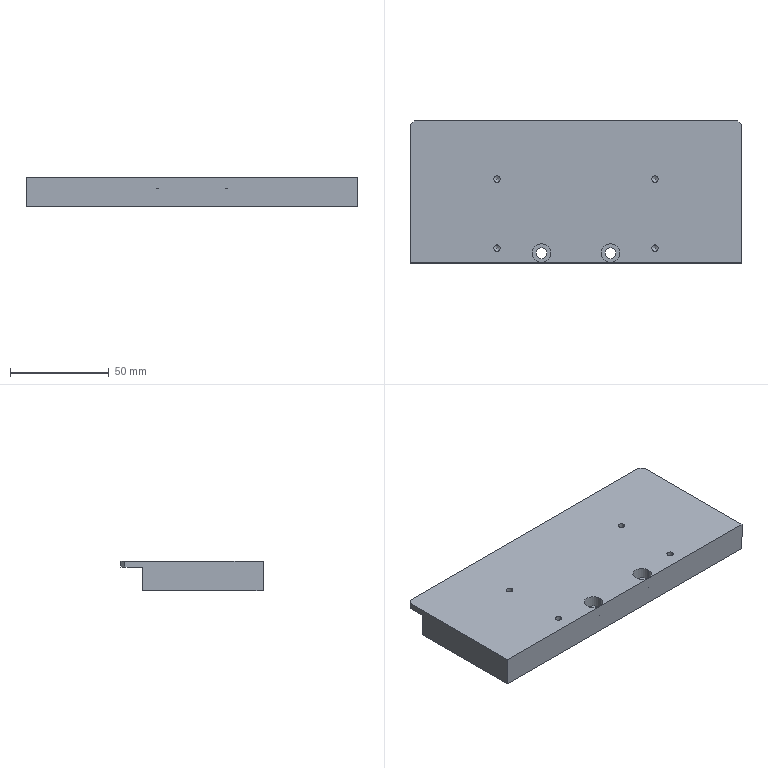Part | SolidWorks | features HoleWzd 10, ICE 4, Chamfer 2, Cut 1, Extrusion 1, Fillet 1 | 1 solid | 52 faces | box 168 x 72 x 15 mm | volume 156428 mm3 | cylinder 24 | cone 16 | plane 12 | commonest cylinder face diameters 3.3 x8 5 x8 5.5 x4 9.5 x4
STEP:
#1=CARTESIAN_POINT('',(61.75,272.,1.8));
#2=VERTEX_POINT('',#1);
#3=CARTESIAN_POINT('',(71.25,272.,1.8));
#4=VERTEX_POINT('',#3);
#5=CARTESIAN_POINT('',(66.5,272.,1.8));
#6=DIRECTION('',(0.,0.,1.));
#7=DIRECTION('',(1.,0.,0.));
#8=AXIS2_PLACEMENT_3D('',#5,#6,#7);
#9=CIRCLE('',#8,4.75);
#10=EDGE_CURVE('',#2,#4,#9,.T.);
#11=ORIENTED_EDGE('',*,*,#10,.F.);
#12=CARTESIAN_POINT('',(61.75,272.,7.5));
#13=VERTEX_POINT('',#12);
#14=CARTESIAN_POINT('',(61.75,272.,7.5));
#15=DIRECTION('',(0.,0.,1.));
#16=VECTOR('',#15,1000.);
#17=LINE('',#14,#16);
#18=EDGE_CURVE('',#2,#13,#17,.T.);
#19=ORIENTED_EDGE('',*,*,#18,.T.);
#20=CARTESIAN_POINT('',(71.25,272.,7.5));
#21=VERTEX_POINT('',#20);
#22=CARTESIAN_POINT('',(66.5,272.,7.5));
#23=DIRECTION('',(0.,0.,1.));
#24=DIRECTION('',(1.,0.,0.));
#25=AXIS2_PLACEMENT_3D('',#22,#23,#24);
#26=CIRCLE('',#25,4.75);
#27=EDGE_CURVE('',#13,#21,#26,.T.);
#28=ORIENTED_EDGE('',*,*,#27,.T.);
#29=CARTESIAN_POINT('',(71.25,272.,7.5));
#30=DIRECTION('',(0.,0.,1.));
#31=VECTOR('',#30,1000.);
#32=LINE('',#29,#31);
#33=EDGE_CURVE('',#4,#21,#32,.T.);
#34=ORIENTED_EDGE('',*,*,#33,.F.);
#35=EDGE_LOOP('',(#11,#19,#28,#34));
#36=FACE_OUTER_BOUND('',#35,.T.);
#37=CARTESIAN_POINT('',(66.5,272.,7.5));
#38=DIRECTION('',(0.,0.,1.));
#39=DIRECTION('',(1.,0.,0.));
#40=AXIS2_PLACEMENT_3D('',#37,#38,#39);
#41=CYLINDRICAL_SURFACE('',#40,4.75);
#42=ADVANCED_FACE('',(#36),#41,.F.);
#43=CARTESIAN_POINT('',(63.75,272.,-7.5));
#44=VERTEX_POINT('',#43);
#45=CARTESIAN_POINT('',(69.25,272.,-7.5));
#46=VERTEX_POINT('',#45);
#47=CARTESIAN_POINT('',(66.5,272.,-7.5));
#48=DIRECTION('',(0.,0.,1.));
#49=DIRECTION('',(1.,0.,0.));
#50=AXIS2_PLACEMENT_3D('',#47,#48,#49);
#51=CIRCLE('',#50,2.75);
#52=EDGE_CURVE('',#44,#46,#51,.T.);
#53=ORIENTED_EDGE('',*,*,#52,.F.);
#54=CARTESIAN_POINT('',(63.75,272.,1.8));
#55=VERTEX_POINT('',#54);
#56=CARTESIAN_POINT('',(63.75,272.,7.5));
#57=DIRECTION('',(0.,0.,1.));
#58=VECTOR('',#57,1000.);
#59=LINE('',#56,#58);
#60=EDGE_CURVE('',#44,#55,#59,.T.);
#61=ORIENTED_EDGE('',*,*,#60,.T.);
#62=CARTESIAN_POINT('',(69.25,272.,1.8));
#63=VERTEX_POINT('',#62);
#64=CARTESIAN_POINT('',(66.5,272.,1.8));
#65=DIRECTION('',(0.,0.,1.));
#66=DIRECTION('',(1.,0.,0.));
#67=AXIS2_PLACEMENT_3D('',#64,#65,#66);
#68=CIRCLE('',#67,2.75);
#69=EDGE_CURVE('',#55,#63,#68,.T.);
#70=ORIENTED_EDGE('',*,*,#69,.T.);
#71=CARTESIAN_POINT('',(69.25,272.,7.5));
#72=DIRECTION('',(0.,0.,1.));
#73=VECTOR('',#72,1000.);
#74=LINE('',#71,#73);
#75=EDGE_CURVE('',#46,#63,#74,.T.);
#76=ORIENTED_EDGE('',*,*,#75,.F.);
#77=EDGE_LOOP('',(#53,#61,#70,#76));
#78=FACE_OUTER_BOUND('',#77,.T.);
#79=CARTESIAN_POINT('',(66.5,272.,7.5));
#80=DIRECTION('',(0.,0.,1.));
#81=DIRECTION('',(1.,0.,0.));
#82=AXIS2_PLACEMENT_3D('',#79,#80,#81);
#83=CYLINDRICAL_SURFACE('',#82,2.75);
#84=ADVANCED_FACE('',(#78),#83,.F.);
#85=CARTESIAN_POINT('',(96.75,272.,1.8));
#86=VERTEX_POINT('',#85);
#87=CARTESIAN_POINT('',(106.25,272.,1.8));
#88=VERTEX_POINT('',#87);
#89=CARTESIAN_POINT('',(101.5,272.,1.8));
#90=DIRECTION('',(0.,0.,1.));
#91=DIRECTION('',(1.,0.,0.));
#92=AXIS2_PLACEMENT_3D('',#89,#90,#91);
#93=CIRCLE('',#92,4.75);
#94=EDGE_CURVE('',#86,#88,#93,.T.);
#95=ORIENTED_EDGE('',*,*,#94,.F.);
#96=CARTESIAN_POINT('',(96.75,272.,7.5));
#97=VERTEX_POINT('',#96);
#98=CARTESIAN_POINT('',(96.75,272.,7.5));
#99=DIRECTION('',(0.,0.,1.));
#100=VECTOR('',#99,1000.);
#101=LINE('',#98,#100);
#102=EDGE_CURVE('',#86,#97,#101,.T.);
#103=ORIENTED_EDGE('',*,*,#102,.T.);
#104=CARTESIAN_POINT('',(106.25,272.,7.5));
#105=VERTEX_POINT('',#104);
#106=CARTESIAN_POINT('',(101.5,272.,7.5));
#107=DIRECTION('',(0.,0.,1.));
#108=DIRECTION('',(1.,0.,0.));
#109=AXIS2_PLACEMENT_3D('',#106,#107,#108);
#110=CIRCLE('',#109,4.75);
#111=EDGE_CURVE('',#97,#105,#110,.T.);
#112=ORIENTED_EDGE('',*,*,#111,.T.);
#113=CARTESIAN_POINT('',(106.25,272.,7.5));
#114=DIRECTION('',(0.,0.,1.));
#115=VECTOR('',#114,1000.);
#116=LINE('',#113,#115);
#117=EDGE_CURVE('',#88,#105,#116,.T.);
#118=ORIENTED_EDGE('',*,*,#117,.F.);
#119=EDGE_LOOP('',(#95,#103,#112,#118));
#120=FACE_OUTER_BOUND('',#119,.T.);
#121=CARTESIAN_POINT('',(101.5,272.,7.5));
#122=DIRECTION('',(0.,0.,1.));
#123=DIRECTION('',(1.,0.,0.));
#124=AXIS2_PLACEMENT_3D('',#121,#122,#123);
#125=CYLINDRICAL_SURFACE('',#124,4.75);
#126=ADVANCED_FACE('',(#120),#125,.F.);
#127=CARTESIAN_POINT('',(98.75,272.,-7.5));
#128=VERTEX_POINT('',#127);
#129=CARTESIAN_POINT('',(104.25,272.,-7.5));
#130=VERTEX_POINT('',#129);
#131=CARTESIAN_POINT('',(101.5,272.,-7.5));
#132=DIRECTION('',(0.,0.,1.));
#133=DIRECTION('',(1.,0.,0.));
#134=AXIS2_PLACEMENT_3D('',#131,#132,#133);
#135=CIRCLE('',#134,2.75);
#136=EDGE_CURVE('',#128,#130,#135,.T.);
#137=ORIENTED_EDGE('',*,*,#136,.F.);
#138=CARTESIAN_POINT('',(98.75,272.,1.8));
#139=VERTEX_POINT('',#138);
#140=CARTESIAN_POINT('',(98.75,272.,7.5));
#141=DIRECTION('',(0.,0.,1.));
#142=VECTOR('',#141,1000.);
#143=LINE('',#140,#142);
#144=EDGE_CURVE('',#128,#139,#143,.T.);
#145=ORIENTED_EDGE('',*,*,#144,.T.);
#146=CARTESIAN_POINT('',(104.25,272.,1.8));
#147=VERTEX_POINT('',#146);
#148=CARTESIAN_POINT('',(101.5,272.,1.8));
#149=DIRECTION('',(0.,0.,1.));
#150=DIRECTION('',(1.,0.,0.));
#151=AXIS2_PLACEMENT_3D('',#148,#149,#150);
#152=CIRCLE('',#151,2.75);
#153=EDGE_CURVE('',#139,#147,#152,.T.);
#154=ORIENTED_EDGE('',*,*,#153,.T.);
#155=CARTESIAN_POINT('',(104.25,272.,7.5));
#156=DIRECTION('',(0.,0.,1.));
#157=VECTOR('',#156,1000.);
#158=LINE('',#155,#157);
#159=EDGE_CURVE('',#130,#147,#158,.T.);
#160=ORIENTED_EDGE('',*,*,#159,.F.);
#161=EDGE_LOOP('',(#137,#145,#154,#160));
#162=FACE_OUTER_BOUND('',#161,.T.);
#163=CARTESIAN_POINT('',(101.5,272.,7.5));
#164=DIRECTION('',(0.,0.,1.));
#165=DIRECTION('',(1.,0.,0.));
#166=AXIS2_PLACEMENT_3D('',#163,#164,#165);
#167=CYLINDRICAL_SURFACE('',#166,2.75);
#168=ADVANCED_FACE('',(#162),#167,.F.);
#169=CARTESIAN_POINT('',(42.35,309.5,-2.6));
#170=VERTEX_POINT('',#169);
#171=CARTESIAN_POINT('',(45.65,309.5,-2.6));
#172=VERTEX_POINT('',#171);
#173=CARTESIAN_POINT('',(44.,309.5,-2.6));
#174=DIRECTION('',(0.,0.,1.));
#175=DIRECTION('',(1.,0.,0.));
#176=AXIS2_PLACEMENT_3D('',#173,#174,#175);
#177=CIRCLE('',#176,1.65);
#178=EDGE_CURVE('',#170,#172,#177,.T.);
#179=ORIENTED_EDGE('',*,*,#178,.F.);
#180=CARTESIAN_POINT('',(42.35,309.5,7.5));
#181=VERTEX_POINT('',#180);
#182=CARTESIAN_POINT('',(42.35,309.5,7.5));
#183=DIRECTION('',(0.,0.,1.));
#184=VECTOR('',#183,1000.);
#185=LINE('',#182,#184);
#186=EDGE_CURVE('',#170,#181,#185,.T.);
#187=ORIENTED_EDGE('',*,*,#186,.T.);
#188=CARTESIAN_POINT('',(45.65,309.5,7.5));
#189=VERTEX_POINT('',#188);
#190=CARTESIAN_POINT('',(44.,309.5,7.5));
#191=DIRECTION('',(0.,0.,1.));
#192=DIRECTION('',(1.,0.,0.));
#193=AXIS2_PLACEMENT_3D('',#190,#191,#192);
#194=CIRCLE('',#193,1.65);
#195=EDGE_CURVE('',#181,#189,#194,.T.);
#196=ORIENTED_EDGE('',*,*,#195,.T.);
#197=CARTESIAN_POINT('',(45.65,309.5,7.5));
#198=DIRECTION('',(0.,0.,1.));
#199=VECTOR('',#198,1000.);
#200=LINE('',#197,#199);
#201=EDGE_CURVE('',#172,#189,#200,.T.);
#202=ORIENTED_EDGE('',*,*,#201,.F.);
#203=EDGE_LOOP('',(#179,#187,#196,#202));
#204=FACE_OUTER_BOUND('',#203,.T.);
#205=CARTESIAN_POINT('',(44.,309.5,7.5));
#206=DIRECTION('',(0.,0.,1.));
#207=DIRECTION('',(1.,0.,0.));
#208=AXIS2_PLACEMENT_3D('',#205,#206,#207);
#209=CYLINDRICAL_SURFACE('',#208,1.65);
#210=ADVANCED_FACE('',(#204),#209,.F.);
#211=CARTESIAN_POINT('',(44.,309.5,-3.591));
#212=VERTEX_POINT('',#211);
#213=CARTESIAN_POINT('',(45.65,309.5,-2.6));
#214=DIRECTION('',(0.8572,0.,0.515));
#215=VECTOR('',#214,1000.);
#216=LINE('',#213,#215);
#217=EDGE_CURVE('',#212,#172,#216,.T.);
#218=ORIENTED_EDGE('',*,*,#217,.F.);
#219=CARTESIAN_POINT('',(42.35,309.5,-2.6));
#220=DIRECTION('',(-0.8572,0.,0.515));
#221=VECTOR('',#220,1000.);
#222=LINE('',#219,#221);
#223=EDGE_CURVE('',#212,#170,#222,.T.);
#224=ORIENTED_EDGE('',*,*,#223,.T.);
#225=ORIENTED_EDGE('',*,*,#178,.T.);
#226=EDGE_LOOP('',(#218,#224,#225));
#227=FACE_OUTER_BOUND('',#226,.T.);
#228=CARTESIAN_POINT('',(44.,309.5,-2.6));
#229=DIRECTION('',(0.,0.,1.));
#230=DIRECTION('',(1.,0.,0.));
#231=AXIS2_PLACEMENT_3D('',#228,#229,#230);
#232=CONICAL_SURFACE('',#231,1.65,1.03);
#233=ADVANCED_FACE('',(#227),#232,.F.);
#234=CARTESIAN_POINT('',(42.35,274.5,-2.6));
#235=VERTEX_POINT('',#234);
#236=CARTESIAN_POINT('',(45.65,274.5,-2.6));
#237=VERTEX_POINT('',#236);
#238=CARTESIAN_POINT('',(44.,274.5,-2.6));
#239=DIRECTION('',(0.,0.,1.));
#240=DIRECTION('',(1.,0.,0.));
#241=AXIS2_PLACEMENT_3D('',#238,#239,#240);
#242=CIRCLE('',#241,1.65);
#243=EDGE_CURVE('',#235,#237,#242,.T.);
#244=ORIENTED_EDGE('',*,*,#243,.F.);
#245=CARTESIAN_POINT('',(42.35,274.5,7.5));
#246=VERTEX_POINT('',#245);
#247=CARTESIAN_POINT('',(42.35,274.5,7.5));
#248=DIRECTION('',(0.,0.,1.));
#249=VECTOR('',#248,1000.);
#250=LINE('',#247,#249);
#251=EDGE_CURVE('',#235,#246,#250,.T.);
#252=ORIENTED_EDGE('',*,*,#251,.T.);
#253=CARTESIAN_POINT('',(45.65,274.5,7.5));
#254=VERTEX_POINT('',#253);
#255=CARTESIAN_POINT('',(44.,274.5,7.5));
#256=DIRECTION('',(0.,0.,1.));
#257=DIRECTION('',(1.,0.,0.));
#258=AXIS2_PLACEMENT_3D('',#255,#256,#257);
#259=CIRCLE('',#258,1.65);
#260=EDGE_CURVE('',#246,#254,#259,.T.);
#261=ORIENTED_EDGE('',*,*,#260,.T.);
#262=CARTESIAN_POINT('',(45.65,274.5,7.5));
#263=DIRECTION('',(0.,0.,1.));
#264=VECTOR('',#263,1000.);
#265=LINE('',#262,#264);
#266=EDGE_CURVE('',#237,#254,#265,.T.);
#267=ORIENTED_EDGE('',*,*,#266,.F.);
#268=EDGE_LOOP('',(#244,#252,#261,#267));
#269=FACE_OUTER_BOUND('',#268,.T.);
#270=CARTESIAN_POINT('',(44.,274.5,7.5));
#271=DIRECTION('',(0.,0.,1.));
#272=DIRECTION('',(1.,0.,0.));
#273=AXIS2_PLACEMENT_3D('',#270,#271,#272);
#274=CYLINDRICAL_SURFACE('',#273,1.65);
#275=ADVANCED_FACE('',(#269),#274,.F.);
#276=CARTESIAN_POINT('',(44.,274.5,-3.591));
#277=VERTEX_POINT('',#276);
#278=CARTESIAN_POINT('',(45.65,274.5,-2.6));
#279=DIRECTION('',(0.8572,0.,0.515));
#280=VECTOR('',#279,1000.);
#281=LINE('',#278,#280);
#282=EDGE_CURVE('',#277,#237,#281,.T.);
#283=ORIENTED_EDGE('',*,*,#282,.F.);
#284=CARTESIAN_POINT('',(42.35,274.5,-2.6));
#285=DIRECTION('',(-0.8572,0.,0.515));
#286=VECTOR('',#285,1000.);
#287=LINE('',#284,#286);
#288=EDGE_CURVE('',#277,#235,#287,.T.);
#289=ORIENTED_EDGE('',*,*,#288,.T.);
#290=ORIENTED_EDGE('',*,*,#243,.T.);
#291=EDGE_LOOP('',(#283,#289,#290));
#292=FACE_OUTER_BOUND('',#291,.T.);
#293=CARTESIAN_POINT('',(44.,274.5,-2.6));
#294=DIRECTION('',(0.,0.,1.));
#295=DIRECTION('',(1.,0.,0.));
#296=AXIS2_PLACEMENT_3D('',#293,#294,#295);
#297=CONICAL_SURFACE('',#296,1.65,1.03);
#298=ADVANCED_FACE('',(#292),#297,.F.);
#299=CARTESIAN_POINT('',(122.35,274.5,-2.6));
#300=VERTEX_POINT('',#299);
#301=CARTESIAN_POINT('',(125.65,274.5,-2.6));
#302=VERTEX_POINT('',#301);
#303=CARTESIAN_POINT('',(124.,274.5,-2.6));
#304=DIRECTION('',(0.,0.,1.));
#305=DIRECTION('',(1.,0.,0.));
#306=AXIS2_PLACEMENT_3D('',#303,#304,#305);
#307=CIRCLE('',#306,1.65);
#308=EDGE_CURVE('',#300,#302,#307,.T.);
#309=ORIENTED_EDGE('',*,*,#308,.F.);
#310=CARTESIAN_POINT('',(122.35,274.5,7.5));
#311=VERTEX_POINT('',#310);
#312=CARTESIAN_POINT('',(122.35,274.5,7.5));
#313=DIRECTION('',(0.,0.,1.));
#314=VECTOR('',#313,1000.);
#315=LINE('',#312,#314);
#316=EDGE_CURVE('',#300,#311,#315,.T.);
#317=ORIENTED_EDGE('',*,*,#316,.T.);
#318=CARTESIAN_POINT('',(125.65,274.5,7.5));
#319=VERTEX_POINT('',#318);
#320=CARTESIAN_POINT('',(124.,274.5,7.5));
#321=DIRECTION('',(0.,0.,1.));
#322=DIRECTION('',(1.,0.,0.));
#323=AXIS2_PLACEMENT_3D('',#320,#321,#322);
#324=CIRCLE('',#323,1.65);
#325=EDGE_CURVE('',#311,#319,#324,.T.);
#326=ORIENTED_EDGE('',*,*,#325,.T.);
#327=CARTESIAN_POINT('',(125.65,274.5,7.5));
#328=DIRECTION('',(0.,0.,1.));
#329=VECTOR('',#328,1000.);
#330=LINE('',#327,#329);
#331=EDGE_CURVE('',#302,#319,#330,.T.);
#332=ORIENTED_EDGE('',*,*,#331,.F.);
#333=EDGE_LOOP('',(#309,#317,#326,#332));
#334=FACE_OUTER_BOUND('',#333,.T.);
#335=CARTESIAN_POINT('',(124.,274.5,7.5));
#336=DIRECTION('',(0.,0.,1.));
#337=DIRECTION('',(1.,0.,0.));
#338=AXIS2_PLACEMENT_3D('',#335,#336,#337);
#339=CYLINDRICAL_SURFACE('',#338,1.65);
#340=ADVANCED_FACE('',(#334),#339,.F.);
#341=CARTESIAN_POINT('',(124.,274.5,-3.591));
#342=VERTEX_POINT('',#341);
#343=CARTESIAN_POINT('',(125.65,274.5,-2.6));
#344=DIRECTION('',(0.8572,0.,0.515));
#345=VECTOR('',#344,1000.);
#346=LINE('',#343,#345);
#347=EDGE_CURVE('',#342,#302,#346,.T.);
#348=ORIENTED_EDGE('',*,*,#347,.F.);
#349=CARTESIAN_POINT('',(122.35,274.5,-2.6));
#350=DIRECTION('',(-0.8572,0.,0.515));
#351=VECTOR('',#350,1000.);
#352=LINE('',#349,#351);
#353=EDGE_CURVE('',#342,#300,#352,.T.);
#354=ORIENTED_EDGE('',*,*,#353,.T.);
#355=ORIENTED_EDGE('',*,*,#308,.T.);
#356=EDGE_LOOP('',(#348,#354,#355));
#357=FACE_OUTER_BOUND('',#356,.T.);
#358=CARTESIAN_POINT('',(124.,274.5,-2.6));
#359=DIRECTION('',(0.,0.,1.));
#360=DIRECTION('',(1.,0.,0.));
#361=AXIS2_PLACEMENT_3D('',#358,#359,#360);
#362=CONICAL_SURFACE('',#361,1.65,1.03);
#363=ADVANCED_FACE('',(#357),#362,.F.);
#364=CARTESIAN_POINT('',(122.35,309.5,-2.6));
#365=VERTEX_POINT('',#364);
#366=CARTESIAN_POINT('',(125.65,309.5,-2.6));
#367=VERTEX_POINT('',#366);
#368=CARTESIAN_POINT('',(124.,309.5,-2.6));
#369=DIRECTION('',(0.,0.,1.));
#370=DIRECTION('',(1.,0.,0.));
#371=AXIS2_PLACEMENT_3D('',#368,#369,#370);
#372=CIRCLE('',#371,1.65);
#373=EDGE_CURVE('',#365,#367,#372,.T.);
#374=ORIENTED_EDGE('',*,*,#373,.F.);
#375=CARTESIAN_POINT('',(122.35,309.5,7.5));
#376=VERTEX_POINT('',#375);
#377=CARTESIAN_POINT('',(122.35,309.5,7.5));
#378=DIRECTION('',(0.,0.,1.));
#379=VECTOR('',#378,1000.);
#380=LINE('',#377,#379);
#381=EDGE_CURVE('',#365,#376,#380,.T.);
#382=ORIENTED_EDGE('',*,*,#381,.T.);
#383=CARTESIAN_POINT('',(125.65,309.5,7.5));
#384=VERTEX_POINT('',#383);
#385=CARTESIAN_POINT('',(124.,309.5,7.5));
#386=DIRECTION('',(0.,0.,1.));
#387=DIRECTION('',(1.,0.,0.));
#388=AXIS2_PLACEMENT_3D('',#385,#386,#387);
#389=CIRCLE('',#388,1.65);
#390=EDGE_CURVE('',#376,#384,#389,.T.);
#391=ORIENTED_EDGE('',*,*,#390,.T.);
#392=CARTESIAN_POINT('',(125.65,309.5,7.5));
#393=DIRECTION('',(0.,0.,1.));
#394=VECTOR('',#393,1000.);
#395=LINE('',#392,#394);
#396=EDGE_CURVE('',#367,#384,#395,.T.);
#397=ORIENTED_EDGE('',*,*,#396,.F.);
#398=EDGE_LOOP('',(#374,#382,#391,#397));
#399=FACE_OUTER_BOUND('',#398,.T.);
#400=CARTESIAN_POINT('',(124.,309.5,7.5));
#401=DIRECTION('',(0.,0.,1.));
#402=DIRECTION('',(1.,0.,0.));
#403=AXIS2_PLACEMENT_3D('',#400,#401,#402);
#404=CYLINDRICAL_SURFACE('',#403,1.65);
#405=ADVANCED_FACE('',(#399),#404,.F.);
#406=CARTESIAN_POINT('',(124.,309.5,-3.591));
#407=VERTEX_POINT('',#406);
#408=CARTESIAN_POINT('',(125.65,309.5,-2.6));
#409=DIRECTION('',(0.8572,0.,0.515));
#410=VECTOR('',#409,1000.);
#411=LINE('',#408,#410);
#412=EDGE_CURVE('',#407,#367,#411,.T.);
#413=ORIENTED_EDGE('',*,*,#412,.F.);
#414=CARTESIAN_POINT('',(122.35,309.5,-2.6));
#415=DIRECTION('',(-0.8572,0.,0.515));
#416=VECTOR('',#415,1000.);
#417=LINE('',#414,#416);
#418=EDGE_CURVE('',#407,#365,#417,.T.);
#419=ORIENTED_EDGE('',*,*,#418,.T.);
#420=ORIENTED_EDGE('',*,*,#373,.T.);
#421=EDGE_LOOP('',(#413,#419,#420));
#422=FACE_OUTER_BOUND('',#421,.T.);
#423=CARTESIAN_POINT('',(124.,309.5,-2.6));
#424=DIRECTION('',(0.,0.,1.));
#425=DIRECTION('',(1.,0.,0.));
#426=AXIS2_PLACEMENT_3D('',#423,#424,#425);
#427=CONICAL_SURFACE('',#426,1.65,1.03);
#428=ADVANCED_FACE('',(#422),#427,.F.);
#429=CARTESIAN_POINT('',(151.5,313.,-4.));
#430=VERTEX_POINT('',#429);
#431=CARTESIAN_POINT('',(151.5,313.,1.));
#432=VERTEX_POINT('',#431);
#433=CARTESIAN_POINT('',(151.5,313.,-1.5));
#434=DIRECTION('',(0.,1.,0.));
#435=DIRECTION('',(0.,0.,1.));
#436=AXIS2_PLACEMENT_3D('',#433,#434,#435);
#437=CIRCLE('',#436,2.5);
#438=EDGE_CURVE('',#430,#432,#437,.T.);
#439=ORIENTED_EDGE('',*,*,#438,.F.);
#440=CARTESIAN_POINT('',(151.5,328.,-4.));
#441=VERTEX_POINT('',#440);
#442=CARTESIAN_POINT('',(151.5,328.,-4.));
#443=DIRECTION('',(0.,1.,0.));
#444=VECTOR('',#443,1000.);
#445=LINE('',#442,#444);
#446=EDGE_CURVE('',#430,#441,#445,.T.);
#447=ORIENTED_EDGE('',*,*,#446,.T.);
#448=CARTESIAN_POINT('',(151.5,328.,1.));
#449=VERTEX_POINT('',#448);
#450=CARTESIAN_POINT('',(151.5,328.,-1.5));
#451=DIRECTION('',(0.,1.,0.));
#452=DIRECTION('',(0.,0.,1.));
#453=AXIS2_PLACEMENT_3D('',#450,#451,#452);
#454=CIRCLE('',#453,2.5);
#455=EDGE_CURVE('',#441,#449,#454,.T.);
#456=ORIENTED_EDGE('',*,*,#455,.T.);
#457=CARTESIAN_POINT('',(151.5,328.,1.));
#458=DIRECTION('',(0.,1.,0.));
#459=VECTOR('',#458,1000.);
#460=LINE('',#457,#459);
#461=EDGE_CURVE('',#432,#449,#460,.T.);
#462=ORIENTED_EDGE('',*,*,#461,.F.);
#463=EDGE_LOOP('',(#439,#447,#456,#462));
#464=FACE_OUTER_BOUND('',#463,.T.);
#465=CARTESIAN_POINT('',(151.5,328.,-1.5));
#466=DIRECTION('',(0.,1.,0.));
#467=DIRECTION('',(0.,0.,1.));
#468=AXIS2_PLACEMENT_3D('',#465,#466,#467);
#469=CYLINDRICAL_SURFACE('',#468,2.5);
#470=ADVANCED_FACE('',(#464),#469,.F.);
#471=CARTESIAN_POINT('',(151.5,311.498,-1.5));
#472=VERTEX_POINT('',#471);
#473=CARTESIAN_POINT('',(151.5,313.,1.));
#474=DIRECTION('',(0.,0.515,0.8572));
#475=VECTOR('',#474,1000.);
#476=LINE('',#473,#475);
#477=EDGE_CURVE('',#472,#432,#476,.T.);
#478=ORIENTED_EDGE('',*,*,#477,.F.);
#479=CARTESIAN_POINT('',(151.5,313.,-4.));
#480=DIRECTION('',(0.,0.515,-0.8572));
#481=VECTOR('',#480,1000.);
#482=LINE('',#479,#481);
#483=EDGE_CURVE('',#472,#430,#482,.T.);
#484=ORIENTED_EDGE('',*,*,#483,.T.);
#485=ORIENTED_EDGE('',*,*,#438,.T.);
#486=EDGE_LOOP('',(#478,#484,#485));
#487=FACE_OUTER_BOUND('',#486,.T.);
#488=CARTESIAN_POINT('',(151.5,313.,-1.5));
#489=DIRECTION('',(0.,1.,0.));
#490=DIRECTION('',(0.,0.,1.));
#491=AXIS2_PLACEMENT_3D('',#488,#489,#490);
#492=CONICAL_SURFACE('',#491,2.5,1.03);
#493=ADVANCED_FACE('',(#487),#492,.F.);
#494=CARTESIAN_POINT('',(106.5,313.,-4.));
#495=VERTEX_POINT('',#494);
#496=CARTESIAN_POINT('',(106.5,313.,1.));
#497=VERTEX_POINT('',#496);
#498=CARTESIAN_POINT('',(106.5,313.,-1.5));
#499=DIRECTION('',(0.,1.,0.));
#500=DIRECTION('',(0.,0.,1.));
#501=AXIS2_PLACEMENT_3D('',#498,#499,#500);
#502=CIRCLE('',#501,2.5);
#503=EDGE_CURVE('',#495,#497,#502,.T.);
#504=ORIENTED_EDGE('',*,*,#503,.F.);
#505=CARTESIAN_POINT('',(106.5,328.,-4.));
#506=VERTEX_POINT('',#505);
#507=CARTESIAN_POINT('',(106.5,328.,-4.));
#508=DIRECTION('',(0.,1.,0.));
#509=VECTOR('',#508,1000.);
#510=LINE('',#507,#509);
#511=EDGE_CURVE('',#495,#506,#510,.T.);
#512=ORIENTED_EDGE('',*,*,#511,.T.);
#513=CARTESIAN_POINT('',(106.5,328.,1.));
#514=VERTEX_POINT('',#513);
#515=CARTESIAN_POINT('',(106.5,328.,-1.5));
#516=DIRECTION('',(0.,1.,0.));
#517=DIRECTION('',(0.,0.,1.));
#518=AXIS2_PLACEMENT_3D('',#515,#516,#517);
#519=CIRCLE('',#518,2.5);
#520=EDGE_CURVE('',#506,#514,#519,.T.);
#521=ORIENTED_EDGE('',*,*,#520,.T.);
#522=CARTESIAN_POINT('',(106.5,328.,1.));
#523=DIRECTION('',(0.,1.,0.));
#524=VECTOR('',#523,1000.);
#525=LINE('',#522,#524);
#526=EDGE_CURVE('',#497,#514,#525,.T.);
#527=ORIENTED_EDGE('',*,*,#526,.F.);
#528=EDGE_LOOP('',(#504,#512,#521,#527));
#529=FACE_OUTER_BOUND('',#528,.T.);
#530=CARTESIAN_POINT('',(106.5,328.,-1.5));
#531=DIRECTION('',(0.,1.,0.));
#532=DIRECTION('',(0.,0.,1.));
#533=AXIS2_PLACEMENT_3D('',#530,#531,#532);
#534=CYLINDRICAL_SURFACE('',#533,2.5);
#535=ADVANCED_FACE('',(#529),#534,.F.);
#536=CARTESIAN_POINT('',(106.5,311.498,-1.5));
#537=VERTEX_POINT('',#536);
#538=CARTESIAN_POINT('',(106.5,313.,1.));
#539=DIRECTION('',(0.,0.515,0.8572));
#540=VECTOR('',#539,1000.);
#541=LINE('',#538,#540);
#542=EDGE_CURVE('',#537,#497,#541,.T.);
#543=ORIENTED_EDGE('',*,*,#542,.F.);
#544=CARTESIAN_POINT('',(106.5,313.,-4.));
#545=DIRECTION('',(0.,0.515,-0.8572));
#546=VECTOR('',#545,1000.);
#547=LINE('',#544,#546);
#548=EDGE_CURVE('',#537,#495,#547,.T.);
#549=ORIENTED_EDGE('',*,*,#548,.T.);
#550=ORIENTED_EDGE('',*,*,#503,.T.);
#551=EDGE_LOOP('',(#543,#549,#550));
#552=FACE_OUTER_BOUND('',#551,.T.);
#553=CARTESIAN_POINT('',(106.5,313.,-1.5));
#554=DIRECTION('',(0.,1.,0.));
#555=DIRECTION('',(0.,0.,1.));
#556=AXIS2_PLACEMENT_3D('',#553,#554,#555);
#557=CONICAL_SURFACE('',#556,2.5,1.03);
#558=ADVANCED_FACE('',(#552),#557,.F.);
#559=CARTESIAN_POINT('',(61.5,313.,-4.));
#560=VERTEX_POINT('',#559);
#561=CARTESIAN_POINT('',(61.5,313.,1.));
#562=VERTEX_POINT('',#561);
#563=CARTESIAN_POINT('',(61.5,313.,-1.5));
#564=DIRECTION('',(0.,1.,0.));
#565=DIRECTION('',(0.,0.,1.));
#566=AXIS2_PLACEMENT_3D('',#563,#564,#565);
#567=CIRCLE('',#566,2.5);
#568=EDGE_CURVE('',#560,#562,#567,.T.);
#569=ORIENTED_EDGE('',*,*,#568,.F.);
#570=CARTESIAN_POINT('',(61.5,328.,-4.));
#571=VERTEX_POINT('',#570);
#572=CARTESIAN_POINT('',(61.5,328.,-4.));
#573=DIRECTION('',(0.,1.,0.));
#574=VECTOR('',#573,1000.);
#575=LINE('',#572,#574);
#576=EDGE_CURVE('',#560,#571,#575,.T.);
#577=ORIENTED_EDGE('',*,*,#576,.T.);
#578=CARTESIAN_POINT('',(61.5,328.,1.));
#579=VERTEX_POINT('',#578);
#580=CARTESIAN_POINT('',(61.5,328.,-1.5));
#581=DIRECTION('',(0.,1.,0.));
#582=DIRECTION('',(0.,0.,1.));
#583=AXIS2_PLACEMENT_3D('',#580,#581,#582);
#584=CIRCLE('',#583,2.5);
#585=EDGE_CURVE('',#571,#579,#584,.T.);
#586=ORIENTED_EDGE('',*,*,#585,.T.);
#587=CARTESIAN_POINT('',(61.5,328.,1.));
#588=DIRECTION('',(0.,1.,0.));
#589=VECTOR('',#588,1000.);
#590=LINE('',#587,#589);
#591=EDGE_CURVE('',#562,#579,#590,.T.);
#592=ORIENTED_EDGE('',*,*,#591,.F.);
#593=EDGE_LOOP('',(#569,#577,#586,#592));
#594=FACE_OUTER_BOUND('',#593,.T.);
#595=CARTESIAN_POINT('',(61.5,328.,-1.5));
#596=DIRECTION('',(0.,1.,0.));
#597=DIRECTION('',(0.,0.,1.));
#598=AXIS2_PLACEMENT_3D('',#595,#596,#597);
#599=CYLINDRICAL_SURFACE('',#598,2.5);
#600=ADVANCED_FACE('',(#594),#599,.F.);
#601=CARTESIAN_POINT('',(61.5,311.498,-1.5));
#602=VERTEX_POINT('',#601);
#603=CARTESIAN_POINT('',(61.5,313.,1.));
#604=DIRECTION('',(0.,0.515,0.8572));
#605=VECTOR('',#604,1000.);
#606=LINE('',#603,#605);
#607=EDGE_CURVE('',#602,#562,#606,.T.);
#608=ORIENTED_EDGE('',*,*,#607,.F.);
#609=CARTESIAN_POINT('',(61.5,313.,-4.));
#610=DIRECTION('',(0.,0.515,-0.8572));
#611=VECTOR('',#610,1000.);
#612=LINE('',#609,#611);
#613=EDGE_CURVE('',#602,#560,#612,.T.);
#614=ORIENTED_EDGE('',*,*,#613,.T.);
#615=ORIENTED_EDGE('',*,*,#568,.T.);
#616=EDGE_LOOP('',(#608,#614,#615));
#617=FACE_OUTER_BOUND('',#616,.T.);
#618=CARTESIAN_POINT('',(61.5,313.,-1.5));
#619=DIRECTION('',(0.,1.,0.));
#620=DIRECTION('',(0.,0.,1.));
#621=AXIS2_PLACEMENT_3D('',#618,#619,#620);
#622=CONICAL_SURFACE('',#621,2.5,1.03);
#623=ADVANCED_FACE('',(#617),#622,.F.);
#624=CARTESIAN_POINT('',(16.5,313.,-4.));
#625=VERTEX_POINT('',#624);
#626=CARTESIAN_POINT('',(16.5,313.,1.));
#627=VERTEX_POINT('',#626);
#628=CARTESIAN_POINT('',(16.5,313.,-1.5));
#629=DIRECTION('',(0.,1.,0.));
#630=DIRECTION('',(0.,0.,1.));
#631=AXIS2_PLACEMENT_3D('',#628,#629,#630);
#632=CIRCLE('',#631,2.5);
#633=EDGE_CURVE('',#625,#627,#632,.T.);
#634=ORIENTED_EDGE('',*,*,#633,.F.);
#635=CARTESIAN_POINT('',(16.5,328.,-4.));
#636=VERTEX_POINT('',#635);
#637=CARTESIAN_POINT('',(16.5,328.,-4.));
#638=DIRECTION('',(0.,1.,0.));
#639=VECTOR('',#638,1000.);
#640=LINE('',#637,#639);
#641=EDGE_CURVE('',#625,#636,#640,.T.);
#642=ORIENTED_EDGE('',*,*,#641,.T.);
#643=CARTESIAN_POINT('',(16.5,328.,1.));
#644=VERTEX_POINT('',#643);
#645=CARTESIAN_POINT('',(16.5,328.,-1.5));
#646=DIRECTION('',(0.,1.,0.));
#647=DIRECTION('',(0.,0.,1.));
#648=AXIS2_PLACEMENT_3D('',#645,#646,#647);
#649=CIRCLE('',#648,2.5);
#650=EDGE_CURVE('',#636,#644,#649,.T.);
#651=ORIENTED_EDGE('',*,*,#650,.T.);
#652=CARTESIAN_POINT('',(16.5,328.,1.));
#653=DIRECTION('',(0.,1.,0.));
#654=VECTOR('',#653,1000.);
#655=LINE('',#652,#654);
#656=EDGE_CURVE('',#627,#644,#655,.T.);
#657=ORIENTED_EDGE('',*,*,#656,.F.);
#658=EDGE_LOOP('',(#634,#642,#651,#657));
#659=FACE_OUTER_BOUND('',#658,.T.);
#660=CARTESIAN_POINT('',(16.5,328.,-1.5));
#661=DIRECTION('',(0.,1.,0.));
#662=DIRECTION('',(0.,0.,1.));
#663=AXIS2_PLACEMENT_3D('',#660,#661,#662);
#664=CYLINDRICAL_SURFACE('',#663,2.5);
#665=ADVANCED_FACE('',(#659),#664,.F.);
#666=CARTESIAN_POINT('',(16.5,311.498,-1.5));
#667=VERTEX_POINT('',#666);
#668=CARTESIAN_POINT('',(16.5,313.,1.));
#669=DIRECTION('',(0.,0.515,0.8572));
#670=VECTOR('',#669,1000.);
#671=LINE('',#668,#670);
#672=EDGE_CURVE('',#667,#627,#671,.T.);
#673=ORIENTED_EDGE('',*,*,#672,.F.);
#674=CARTESIAN_POINT('',(16.5,313.,-4.));
#675=DIRECTION('',(0.,0.515,-0.8572));
#676=VECTOR('',#675,1000.);
#677=LINE('',#674,#676);
#678=EDGE_CURVE('',#667,#625,#677,.T.);
#679=ORIENTED_EDGE('',*,*,#678,.T.);
#680=ORIENTED_EDGE('',*,*,#633,.T.);
#681=EDGE_LOOP('',(#673,#679,#680));
#682=FACE_OUTER_BOUND('',#681,.T.);
#683=CARTESIAN_POINT('',(16.5,313.,-1.5));
#684=DIRECTION('',(0.,1.,0.));
#685=DIRECTION('',(0.,0.,1.));
#686=AXIS2_PLACEMENT_3D('',#683,#684,#685);
#687=CONICAL_SURFACE('',#686,2.5,1.03);
#688=ADVANCED_FACE('',(#682),#687,.F.);
#689=CARTESIAN_POINT('',(66.5,272.,-7.5));
#690=DIRECTION('',(0.,0.,1.));
#691=DIRECTION('',(1.,0.,0.));
#692=AXIS2_PLACEMENT_3D('',#689,#690,#691);
#693=CIRCLE('',#692,2.75);
#694=EDGE_CURVE('',#46,#44,#693,.T.);
#695=ORIENTED_EDGE('',*,*,#694,.T.);
#696=ORIENTED_EDGE('',*,*,#52,.T.);
#697=EDGE_LOOP('',(#695,#696));
#698=FACE_BOUND('',#697,.T.);
#699=CARTESIAN_POINT('',(101.5,272.,-7.5));
#700=DIRECTION('',(0.,0.,1.));
#701=DIRECTION('',(1.,0.,0.));
#702=AXIS2_PLACEMENT_3D('',#699,#700,#701);
#703=CIRCLE('',#702,2.75);
#704=EDGE_CURVE('',#130,#128,#703,.T.);
#705=ORIENTED_EDGE('',*,*,#704,.T.);
#706=ORIENTED_EDGE('',*,*,#136,.T.);
#707=EDGE_LOOP('',(#705,#706));
#708=FACE_BOUND('',#707,.T.);
#709=CARTESIAN_POINT('',(168.,267.,-7.5));
#710=VERTEX_POINT('',#709);
#711=CARTESIAN_POINT('',(168.,328.,-7.5));
#712=VERTEX_POINT('',#711);
#713=CARTESIAN_POINT('',(168.,340.,-7.5));
#714=DIRECTION('',(0.,1.,0.));
#715=VECTOR('',#714,1000.);
#716=LINE('',#713,#715);
#717=EDGE_CURVE('',#710,#712,#716,.T.);
#718=ORIENTED_EDGE('',*,*,#717,.F.);
#719=CARTESIAN_POINT('',(0.,267.,-7.5));
#720=VERTEX_POINT('',#719);
#721=CARTESIAN_POINT('',(0.,267.,-7.5));
#722=DIRECTION('',(1.,0.,0.));
#723=VECTOR('',#722,1000.);
#724=LINE('',#721,#723);
#725=EDGE_CURVE('',#720,#710,#724,.T.);
#726=ORIENTED_EDGE('',*,*,#725,.F.);
#727=CARTESIAN_POINT('',(0.,328.,-7.5));
#728=VERTEX_POINT('',#727);
#729=CARTESIAN_POINT('',(0.,0.,-7.5));
#730=DIRECTION('',(0.,-1.,0.));
#731=VECTOR('',#730,1000.);
#732=LINE('',#729,#731);
#733=EDGE_CURVE('',#728,#720,#732,.T.);
#734=ORIENTED_EDGE('',*,*,#733,.F.);
#735=CARTESIAN_POINT('',(0.,328.,-7.5));
#736=DIRECTION('',(-1.,0.,0.));
#737=VECTOR('',#736,1000.);
#738=LINE('',#735,#737);
#739=EDGE_CURVE('',#712,#728,#738,.T.);
#740=ORIENTED_EDGE('',*,*,#739,.F.);
#741=EDGE_LOOP('',(#718,#726,#734,#740));
#742=FACE_OUTER_BOUND('',#741,.T.);
#743=CARTESIAN_POINT('',(0.,0.,-7.5));
#744=DIRECTION('',(0.,0.,-1.));
#745=DIRECTION('',(-1.,0.,0.));
#746=AXIS2_PLACEMENT_3D('',#743,#744,#745);
#747=PLANE('',#746);
#748=ADVANCED_FACE('',(#698,#708,#742),#747,.T.);
#749=CARTESIAN_POINT('',(168.,328.,4.5));
#750=VERTEX_POINT('',#749);
#751=CARTESIAN_POINT('',(168.,337.,4.5));
#752=VERTEX_POINT('',#751);
#753=CARTESIAN_POINT('',(168.,328.,4.5));
#754=DIRECTION('',(0.,1.,0.));
#755=VECTOR('',#754,1000.);
#756=LINE('',#753,#755);
#757=EDGE_CURVE('',#750,#752,#756,.T.);
#758=ORIENTED_EDGE('',*,*,#757,.T.);
#759=CARTESIAN_POINT('',(168.,337.,7.5));
#760=VERTEX_POINT('',#759);
#761=CARTESIAN_POINT('',(168.,337.,7.5));
#762=DIRECTION('',(0.,0.,1.));
#763=VECTOR('',#762,1000.);
#764=LINE('',#761,#763);
#765=EDGE_CURVE('',#752,#760,#764,.T.);
#766=ORIENTED_EDGE('',*,*,#765,.T.);
#767=CARTESIAN_POINT('',(168.,267.,7.5));
#768=VERTEX_POINT('',#767);
#769=CARTESIAN_POINT('',(168.,340.,7.5));
#770=DIRECTION('',(0.,1.,0.));
#771=VECTOR('',#770,1000.);
#772=LINE('',#769,#771);
#773=EDGE_CURVE('',#768,#760,#772,.T.);
#774=ORIENTED_EDGE('',*,*,#773,.F.);
#775=CARTESIAN_POINT('',(168.,267.,7.5));
#776=DIRECTION('',(0.,0.,1.));
#777=VECTOR('',#776,1000.);
#778=LINE('',#775,#777);
#779=EDGE_CURVE('',#710,#768,#778,.T.);
#780=ORIENTED_EDGE('',*,*,#779,.F.);
#781=ORIENTED_EDGE('',*,*,#717,.T.);
#782=CARTESIAN_POINT('',(168.,328.,-7.5));
#783=DIRECTION('',(0.,0.,-1.));
#784=VECTOR('',#783,1000.);
#785=LINE('',#782,#784);
#786=EDGE_CURVE('',#750,#712,#785,.T.);
#787=ORIENTED_EDGE('',*,*,#786,.F.);
#788=EDGE_LOOP('',(#758,#766,#774,#780,#781,#787));
#789=FACE_OUTER_BOUND('',#788,.T.);
#790=CARTESIAN_POINT('',(168.,340.,7.5));
#791=DIRECTION('',(-1.,0.,0.));
#792=DIRECTION('',(0.,-1.,0.));
#793=AXIS2_PLACEMENT_3D('',#790,#791,#792);
#794=PLANE('',#793);
#795=ADVANCED_FACE('',(#789),#794,.F.);
#796=CARTESIAN_POINT('',(0.,337.,7.5));
#797=VERTEX_POINT('',#796);
#798=CARTESIAN_POINT('',(0.,267.,7.5));
#799=VERTEX_POINT('',#798);
#800=CARTESIAN_POINT('',(0.,0.,7.5));
#801=DIRECTION('',(0.,-1.,0.));
#802=VECTOR('',#801,1000.);
#803=LINE('',#800,#802);
#804=EDGE_CURVE('',#797,#799,#803,.T.);
#805=ORIENTED_EDGE('',*,*,#804,.F.);
#806=CARTESIAN_POINT('',(0.,337.,4.5));
#807=VERTEX_POINT('',#806);
#808=CARTESIAN_POINT('',(0.,337.,4.5));
#809=DIRECTION('',(0.,0.,-1.));
#810=VECTOR('',#809,1000.);
#811=LINE('',#808,#810);
#812=EDGE_CURVE('',#797,#807,#811,.T.);
#813=ORIENTED_EDGE('',*,*,#812,.T.);
#814=CARTESIAN_POINT('',(0.,328.,4.5));
#815=VERTEX_POINT('',#814);
#816=CARTESIAN_POINT('',(0.,328.,4.5));
#817=DIRECTION('',(0.,1.,0.));
#818=VECTOR('',#817,1000.);
#819=LINE('',#816,#818);
#820=EDGE_CURVE('',#815,#807,#819,.T.);
#821=ORIENTED_EDGE('',*,*,#820,.F.);
#822=CARTESIAN_POINT('',(0.,328.,-7.5));
#823=DIRECTION('',(0.,0.,1.));
#824=VECTOR('',#823,1000.);
#825=LINE('',#822,#824);
#826=EDGE_CURVE('',#728,#815,#825,.T.);
#827=ORIENTED_EDGE('',*,*,#826,.F.);
#828=ORIENTED_EDGE('',*,*,#733,.T.);
#829=CARTESIAN_POINT('',(0.,267.,-7.5));
#830=DIRECTION('',(0.,0.,1.));
#831=VECTOR('',#830,1000.);
#832=LINE('',#829,#831);
#833=EDGE_CURVE('',#720,#799,#832,.T.);
#834=ORIENTED_EDGE('',*,*,#833,.T.);
#835=EDGE_LOOP('',(#805,#813,#821,#827,#828,#834));
#836=FACE_OUTER_BOUND('',#835,.T.);
#837=CARTESIAN_POINT('',(0.,0.,7.5));
#838=DIRECTION('',(1.,0.,0.));
#839=DIRECTION('',(0.,0.,-1.));
#840=AXIS2_PLACEMENT_3D('',#837,#838,#839);
#841=PLANE('',#840);
#842=ADVANCED_FACE('',(#836),#841,.F.);
#843=CARTESIAN_POINT('',(66.5,272.,7.5));
#844=DIRECTION('',(0.,0.,1.));
#845=DIRECTION('',(1.,0.,0.));
#846=AXIS2_PLACEMENT_3D('',#843,#844,#845);
#847=CIRCLE('',#846,4.75);
#848=EDGE_CURVE('',#21,#13,#847,.T.);
#849=ORIENTED_EDGE('',*,*,#848,.F.);
#850=ORIENTED_EDGE('',*,*,#27,.F.);
#851=EDGE_LOOP('',(#849,#850));
#852=FACE_BOUND('',#851,.T.);
#853=CARTESIAN_POINT('',(101.5,272.,7.5));
#854=DIRECTION('',(0.,0.,1.));
#855=DIRECTION('',(1.,0.,0.));
#856=AXIS2_PLACEMENT_3D('',#853,#854,#855);
#857=CIRCLE('',#856,4.75);
#858=EDGE_CURVE('',#105,#97,#857,.T.);
#859=ORIENTED_EDGE('',*,*,#858,.F.);
#860=ORIENTED_EDGE('',*,*,#111,.F.);
#861=EDGE_LOOP('',(#859,#860));
#862=FACE_BOUND('',#861,.T.);
#863=CARTESIAN_POINT('',(44.,309.5,7.5));
#864=DIRECTION('',(0.,0.,1.));
#865=DIRECTION('',(1.,0.,0.));
#866=AXIS2_PLACEMENT_3D('',#863,#864,#865);
#867=CIRCLE('',#866,1.65);
#868=EDGE_CURVE('',#189,#181,#867,.T.);
#869=ORIENTED_EDGE('',*,*,#868,.F.);
#870=ORIENTED_EDGE('',*,*,#195,.F.);
#871=EDGE_LOOP('',(#869,#870));
#872=FACE_BOUND('',#871,.T.);
#873=CARTESIAN_POINT('',(44.,274.5,7.5));
#874=DIRECTION('',(0.,0.,1.));
#875=DIRECTION('',(1.,0.,0.));
#876=AXIS2_PLACEMENT_3D('',#873,#874,#875);
#877=CIRCLE('',#876,1.65);
#878=EDGE_CURVE('',#254,#246,#877,.T.);
#879=ORIENTED_EDGE('',*,*,#878,.F.);
#880=ORIENTED_EDGE('',*,*,#260,.F.);
#881=EDGE_LOOP('',(#879,#880));
#882=FACE_BOUND('',#881,.T.);
#883=CARTESIAN_POINT('',(124.,274.5,7.5));
#884=DIRECTION('',(0.,0.,1.));
#885=DIRECTION('',(1.,0.,0.));
#886=AXIS2_PLACEMENT_3D('',#883,#884,#885);
#887=CIRCLE('',#886,1.65);
#888=EDGE_CURVE('',#319,#311,#887,.T.);
#889=ORIENTED_EDGE('',*,*,#888,.F.);
#890=ORIENTED_EDGE('',*,*,#325,.F.);
#891=EDGE_LOOP('',(#889,#890));
#892=FACE_BOUND('',#891,.T.);
#893=CARTESIAN_POINT('',(124.,309.5,7.5));
#894=DIRECTION('',(0.,0.,1.));
#895=DIRECTION('',(1.,0.,0.));
#896=AXIS2_PLACEMENT_3D('',#893,#894,#895);
#897=CIRCLE('',#896,1.65);
#898=EDGE_CURVE('',#384,#376,#897,.T.);
#899=ORIENTED_EDGE('',*,*,#898,.F.);
#900=ORIENTED_EDGE('',*,*,#390,.F.);
#901=EDGE_LOOP('',(#899,#900));
#902=FACE_BOUND('',#901,.T.);
#903=CARTESIAN_POINT('',(166.,339.,7.5));
#904=VERTEX_POINT('',#903);
#905=CARTESIAN_POINT('',(2.,339.,7.5));
#906=VERTEX_POINT('',#905);
#907=CARTESIAN_POINT('',(0.,339.,7.5));
#908=DIRECTION('',(-1.,0.,0.));
#909=VECTOR('',#908,1000.);
#910=LINE('',#907,#909);
#911=EDGE_CURVE('',#904,#906,#910,.T.);
#912=ORIENTED_EDGE('',*,*,#911,.T.);
#913=CARTESIAN_POINT('',(0.,337.,7.5));
#914=DIRECTION('',(-0.7071,-0.7071,0.));
#915=VECTOR('',#914,1000.);
#916=LINE('',#913,#915);
#917=EDGE_CURVE('',#906,#797,#916,.T.);
#918=ORIENTED_EDGE('',*,*,#917,.T.);
#919=ORIENTED_EDGE('',*,*,#804,.T.);
#920=CARTESIAN_POINT('',(0.,267.,7.5));
#921=DIRECTION('',(1.,0.,0.));
#922=VECTOR('',#921,1000.);
#923=LINE('',#920,#922);
#924=EDGE_CURVE('',#799,#768,#923,.T.);
#925=ORIENTED_EDGE('',*,*,#924,.T.);
#926=ORIENTED_EDGE('',*,*,#773,.T.);
#927=CARTESIAN_POINT('',(168.,337.,7.5));
#928=DIRECTION('',(-0.7071,0.7071,0.));
#929=VECTOR('',#928,1000.);
#930=LINE('',#927,#929);
#931=EDGE_CURVE('',#760,#904,#930,.T.);
#932=ORIENTED_EDGE('',*,*,#931,.T.);
#933=EDGE_LOOP('',(#912,#918,#919,#925,#926,#932));
#934=FACE_OUTER_BOUND('',#933,.T.);
#935=CARTESIAN_POINT('',(0.,0.,7.5));
#936=DIRECTION('',(0.,0.,-1.));
#937=DIRECTION('',(-1.,0.,0.));
#938=AXIS2_PLACEMENT_3D('',#935,#936,#937);
#939=PLANE('',#938);
#940=ADVANCED_FACE('',(#852,#862,#872,#882,#892,#902,#934),#939,.F.);
#941=ORIENTED_EDGE('',*,*,#820,.T.);
#942=CARTESIAN_POINT('',(2.,339.,4.5));
#943=VERTEX_POINT('',#942);
#944=CARTESIAN_POINT('',(0.,337.,4.5));
#945=DIRECTION('',(0.7071,0.7071,0.));
#946=VECTOR('',#945,1000.);
#947=LINE('',#944,#946);
#948=EDGE_CURVE('',#807,#943,#947,.T.);
#949=ORIENTED_EDGE('',*,*,#948,.T.);
#950=CARTESIAN_POINT('',(166.,339.,4.5));
#951=VERTEX_POINT('',#950);
#952=CARTESIAN_POINT('',(0.,339.,4.5));
#953=DIRECTION('',(-1.,0.,0.));
#954=VECTOR('',#953,1000.);
#955=LINE('',#952,#954);
#956=EDGE_CURVE('',#951,#943,#955,.T.);
#957=ORIENTED_EDGE('',*,*,#956,.F.);
#958=CARTESIAN_POINT('',(168.,337.,4.5));
#959=DIRECTION('',(0.7071,-0.7071,0.));
#960=VECTOR('',#959,1000.);
#961=LINE('',#958,#960);
#962=EDGE_CURVE('',#951,#752,#961,.T.);
#963=ORIENTED_EDGE('',*,*,#962,.T.);
#964=ORIENTED_EDGE('',*,*,#757,.F.);
#965=CARTESIAN_POINT('',(0.,328.,4.5));
#966=DIRECTION('',(1.,0.,0.));
#967=VECTOR('',#966,1000.);
#968=LINE('',#965,#967);
#969=EDGE_CURVE('',#815,#750,#968,.T.);
#970=ORIENTED_EDGE('',*,*,#969,.F.);
#971=EDGE_LOOP('',(#941,#949,#957,#963,#964,#970));
#972=FACE_OUTER_BOUND('',#971,.T.);
#973=CARTESIAN_POINT('',(0.,328.,4.5));
#974=DIRECTION('',(0.,0.,1.));
#975=DIRECTION('',(1.,0.,0.));
#976=AXIS2_PLACEMENT_3D('',#973,#974,#975);
#977=PLANE('',#976);
#978=ADVANCED_FACE('',(#972),#977,.F.);
#979=CARTESIAN_POINT('',(151.5,328.,-1.5));
#980=DIRECTION('',(0.,1.,0.));
#981=DIRECTION('',(0.,0.,1.));
#982=AXIS2_PLACEMENT_3D('',#979,#980,#981);
#983=CIRCLE('',#982,2.5);
#984=EDGE_CURVE('',#449,#441,#983,.T.);
#985=ORIENTED_EDGE('',*,*,#984,.F.);
#986=ORIENTED_EDGE('',*,*,#455,.F.);
#987=EDGE_LOOP('',(#985,#986));
#988=FACE_BOUND('',#987,.T.);
#989=CARTESIAN_POINT('',(106.5,328.,-1.5));
#990=DIRECTION('',(0.,1.,0.));
#991=DIRECTION('',(0.,0.,1.));
#992=AXIS2_PLACEMENT_3D('',#989,#990,#991);
#993=CIRCLE('',#992,2.5);
#994=EDGE_CURVE('',#514,#506,#993,.T.);
#995=ORIENTED_EDGE('',*,*,#994,.F.);
#996=ORIENTED_EDGE('',*,*,#520,.F.);
#997=EDGE_LOOP('',(#995,#996));
#998=FACE_BOUND('',#997,.T.);
#999=CARTESIAN_POINT('',(61.5,328.,-1.5));
#1000=DIRECTION('',(0.,1.,0.));
#1001=DIRECTION('',(0.,0.,1.));
#1002=AXIS2_PLACEMENT_3D('',#999,#1000,#1001);
#1003=CIRCLE('',#1002,2.5);
#1004=EDGE_CURVE('',#579,#571,#1003,.T.);
#1005=ORIENTED_EDGE('',*,*,#1004,.F.);
#1006=ORIENTED_EDGE('',*,*,#585,.F.);
#1007=EDGE_LOOP('',(#1005,#1006));
#1008=FACE_BOUND('',#1007,.T.);
#1009=CARTESIAN_POINT('',(16.5,328.,-1.5));
#1010=DIRECTION('',(0.,1.,0.));
#1011=DIRECTION('',(0.,0.,1.));
#1012=AXIS2_PLACEMENT_3D('',#1009,#1010,#1011);
#1013=CIRCLE('',#1012,2.5);
#1014=EDGE_CURVE('',#644,#636,#1013,.T.);
#1015=ORIENTED_EDGE('',*,*,#1014,.F.);
#1016=ORIENTED_EDGE('',*,*,#650,.F.);
#1017=EDGE_LOOP('',(#1015,#1016));
#1018=FACE_BOUND('',#1017,.T.);
#1019=ORIENTED_EDGE('',*,*,#826,.T.);
#1020=ORIENTED_EDGE('',*,*,#969,.T.);
#1021=ORIENTED_EDGE('',*,*,#786,.T.);
#1022=ORIENTED_EDGE('',*,*,#739,.T.);
#1023=EDGE_LOOP('',(#1019,#1020,#1021,#1022));
#1024=FACE_OUTER_BOUND('',#1023,.T.);
#1025=CARTESIAN_POINT('',(0.,328.,4.5));
#1026=DIRECTION('',(0.,1.,0.));
#1027=DIRECTION('',(0.,0.,1.));
#1028=AXIS2_PLACEMENT_3D('',#1025,#1026,#1027);
#1029=PLANE('',#1028);
#1030=ADVANCED_FACE('',(#988,#998,#1008,#1018,#1024),#1029,.T.);
#1031=ORIENTED_EDGE('',*,*,#678,.F.);
#1032=ORIENTED_EDGE('',*,*,#672,.T.);
#1033=CARTESIAN_POINT('',(16.5,313.,-1.5));
#1034=DIRECTION('',(0.,1.,0.));
#1035=DIRECTION('',(0.,0.,1.));
#1036=AXIS2_PLACEMENT_3D('',#1033,#1034,#1035);
#1037=CIRCLE('',#1036,2.5);
#1038=EDGE_CURVE('',#627,#625,#1037,.T.);
#1039=ORIENTED_EDGE('',*,*,#1038,.T.);
#1040=EDGE_LOOP('',(#1031,#1032,#1039));
#1041=FACE_OUTER_BOUND('',#1040,.T.);
#1042=CARTESIAN_POINT('',(16.5,313.,-1.5));
#1043=DIRECTION('',(0.,1.,0.));
#1044=DIRECTION('',(0.,0.,1.));
#1045=AXIS2_PLACEMENT_3D('',#1042,#1043,#1044);
#1046=CONICAL_SURFACE('',#1045,2.5,1.03);
#1047=ADVANCED_FACE('',(#1041),#1046,.F.);
#1048=ORIENTED_EDGE('',*,*,#641,.F.);
#1049=ORIENTED_EDGE('',*,*,#1038,.F.);
#1050=ORIENTED_EDGE('',*,*,#656,.T.);
#1051=ORIENTED_EDGE('',*,*,#1014,.T.);
#1052=EDGE_LOOP('',(#1048,#1049,#1050,#1051));
#1053=FACE_OUTER_BOUND('',#1052,.T.);
#1054=CARTESIAN_POINT('',(16.5,328.,-1.5));
#1055=DIRECTION('',(0.,1.,0.));
#1056=DIRECTION('',(0.,0.,1.));
#1057=AXIS2_PLACEMENT_3D('',#1054,#1055,#1056);
#1058=CYLINDRICAL_SURFACE('',#1057,2.5);
#1059=ADVANCED_FACE('',(#1053),#1058,.F.);
#1060=ORIENTED_EDGE('',*,*,#613,.F.);
#1061=ORIENTED_EDGE('',*,*,#607,.T.);
#1062=CARTESIAN_POINT('',(61.5,313.,-1.5));
#1063=DIRECTION('',(0.,1.,0.));
#1064=DIRECTION('',(0.,0.,1.));
#1065=AXIS2_PLACEMENT_3D('',#1062,#1063,#1064);
#1066=CIRCLE('',#1065,2.5);
#1067=EDGE_CURVE('',#562,#560,#1066,.T.);
#1068=ORIENTED_EDGE('',*,*,#1067,.T.);
#1069=EDGE_LOOP('',(#1060,#1061,#1068));
#1070=FACE_OUTER_BOUND('',#1069,.T.);
#1071=CARTESIAN_POINT('',(61.5,313.,-1.5));
#1072=DIRECTION('',(0.,1.,0.));
#1073=DIRECTION('',(0.,0.,1.));
#1074=AXIS2_PLACEMENT_3D('',#1071,#1072,#1073);
#1075=CONICAL_SURFACE('',#1074,2.5,1.03);
#1076=ADVANCED_FACE('',(#1070),#1075,.F.);
#1077=ORIENTED_EDGE('',*,*,#576,.F.);
#1078=ORIENTED_EDGE('',*,*,#1067,.F.);
#1079=ORIENTED_EDGE('',*,*,#591,.T.);
#1080=ORIENTED_EDGE('',*,*,#1004,.T.);
#1081=EDGE_LOOP('',(#1077,#1078,#1079,#1080));
#1082=FACE_OUTER_BOUND('',#1081,.T.);
#1083=CARTESIAN_POINT('',(61.5,328.,-1.5));
#1084=DIRECTION('',(0.,1.,0.));
#1085=DIRECTION('',(0.,0.,1.));
#1086=AXIS2_PLACEMENT_3D('',#1083,#1084,#1085);
#1087=CYLINDRICAL_SURFACE('',#1086,2.5);
#1088=ADVANCED_FACE('',(#1082),#1087,.F.);
#1089=ORIENTED_EDGE('',*,*,#548,.F.);
#1090=ORIENTED_EDGE('',*,*,#542,.T.);
#1091=CARTESIAN_POINT('',(106.5,313.,-1.5));
#1092=DIRECTION('',(0.,1.,0.));
#1093=DIRECTION('',(0.,0.,1.));
#1094=AXIS2_PLACEMENT_3D('',#1091,#1092,#1093);
#1095=CIRCLE('',#1094,2.5);
#1096=EDGE_CURVE('',#497,#495,#1095,.T.);
#1097=ORIENTED_EDGE('',*,*,#1096,.T.);
#1098=EDGE_LOOP('',(#1089,#1090,#1097));
#1099=FACE_OUTER_BOUND('',#1098,.T.);
#1100=CARTESIAN_POINT('',(106.5,313.,-1.5));
#1101=DIRECTION('',(0.,1.,0.));
#1102=DIRECTION('',(0.,0.,1.));
#1103=AXIS2_PLACEMENT_3D('',#1100,#1101,#1102);
#1104=CONICAL_SURFACE('',#1103,2.5,1.03);
#1105=ADVANCED_FACE('',(#1099),#1104,.F.);
#1106=ORIENTED_EDGE('',*,*,#511,.F.);
#1107=ORIENTED_EDGE('',*,*,#1096,.F.);
#1108=ORIENTED_EDGE('',*,*,#526,.T.);
#1109=ORIENTED_EDGE('',*,*,#994,.T.);
#1110=EDGE_LOOP('',(#1106,#1107,#1108,#1109));
#1111=FACE_OUTER_BOUND('',#1110,.T.);
#1112=CARTESIAN_POINT('',(106.5,328.,-1.5));
#1113=DIRECTION('',(0.,1.,0.));
#1114=DIRECTION('',(0.,0.,1.));
#1115=AXIS2_PLACEMENT_3D('',#1112,#1113,#1114);
#1116=CYLINDRICAL_SURFACE('',#1115,2.5);
#1117=ADVANCED_FACE('',(#1111),#1116,.F.);
#1118=ORIENTED_EDGE('',*,*,#483,.F.);
#1119=ORIENTED_EDGE('',*,*,#477,.T.);
#1120=CARTESIAN_POINT('',(151.5,313.,-1.5));
#1121=DIRECTION('',(0.,1.,0.));
#1122=DIRECTION('',(0.,0.,1.));
#1123=AXIS2_PLACEMENT_3D('',#1120,#1121,#1122);
#1124=CIRCLE('',#1123,2.5);
#1125=EDGE_CURVE('',#432,#430,#1124,.T.);
#1126=ORIENTED_EDGE('',*,*,#1125,.T.);
#1127=EDGE_LOOP('',(#1118,#1119,#1126));
#1128=FACE_OUTER_BOUND('',#1127,.T.);
#1129=CARTESIAN_POINT('',(151.5,313.,-1.5));
#1130=DIRECTION('',(0.,1.,0.));
#1131=DIRECTION('',(0.,0.,1.));
#1132=AXIS2_PLACEMENT_3D('',#1129,#1130,#1131);
#1133=CONICAL_SURFACE('',#1132,2.5,1.03);
#1134=ADVANCED_FACE('',(#1128),#1133,.F.);
#1135=ORIENTED_EDGE('',*,*,#446,.F.);
#1136=ORIENTED_EDGE('',*,*,#1125,.F.);
#1137=ORIENTED_EDGE('',*,*,#461,.T.);
#1138=ORIENTED_EDGE('',*,*,#984,.T.);
#1139=EDGE_LOOP('',(#1135,#1136,#1137,#1138));
#1140=FACE_OUTER_BOUND('',#1139,.T.);
#1141=CARTESIAN_POINT('',(151.5,328.,-1.5));
#1142=DIRECTION('',(0.,1.,0.));
#1143=DIRECTION('',(0.,0.,1.));
#1144=AXIS2_PLACEMENT_3D('',#1141,#1142,#1143);
#1145=CYLINDRICAL_SURFACE('',#1144,2.5);
#1146=ADVANCED_FACE('',(#1140),#1145,.F.);
#1147=ORIENTED_EDGE('',*,*,#956,.T.);
#1148=CARTESIAN_POINT('',(2.,339.,7.5));
#1149=DIRECTION('',(0.,0.,1.));
#1150=VECTOR('',#1149,1000.);
#1151=LINE('',#1148,#1150);
#1152=EDGE_CURVE('',#943,#906,#1151,.T.);
#1153=ORIENTED_EDGE('',*,*,#1152,.T.);
#1154=ORIENTED_EDGE('',*,*,#911,.F.);
#1155=CARTESIAN_POINT('',(166.,339.,4.5));
#1156=DIRECTION('',(0.,0.,-1.));
#1157=VECTOR('',#1156,1000.);
#1158=LINE('',#1155,#1157);
#1159=EDGE_CURVE('',#904,#951,#1158,.T.);
#1160=ORIENTED_EDGE('',*,*,#1159,.T.);
#1161=EDGE_LOOP('',(#1147,#1153,#1154,#1160));
#1162=FACE_OUTER_BOUND('',#1161,.T.);
#1163=CARTESIAN_POINT('',(0.,339.,-7.5));
#1164=DIRECTION('',(0.,1.,0.));
#1165=DIRECTION('',(0.,0.,1.));
#1166=AXIS2_PLACEMENT_3D('',#1163,#1164,#1165);
#1167=PLANE('',#1166);
#1168=ADVANCED_FACE('',(#1162),#1167,.T.);
#1169=ORIENTED_EDGE('',*,*,#779,.T.);
#1170=ORIENTED_EDGE('',*,*,#924,.F.);
#1171=ORIENTED_EDGE('',*,*,#833,.F.);
#1172=ORIENTED_EDGE('',*,*,#725,.T.);
#1173=EDGE_LOOP('',(#1169,#1170,#1171,#1172));
#1174=FACE_OUTER_BOUND('',#1173,.T.);
#1175=CARTESIAN_POINT('',(0.,267.,-7.5));
#1176=DIRECTION('',(0.,-1.,0.));
#1177=DIRECTION('',(0.,0.,-1.));
#1178=AXIS2_PLACEMENT_3D('',#1175,#1176,#1177);
#1179=PLANE('',#1178);
#1180=ADVANCED_FACE('',(#1174),#1179,.T.);
#1181=ORIENTED_EDGE('',*,*,#418,.F.);
#1182=ORIENTED_EDGE('',*,*,#412,.T.);
#1183=CARTESIAN_POINT('',(124.,309.5,-2.6));
#1184=DIRECTION('',(0.,0.,1.));
#1185=DIRECTION('',(1.,0.,0.));
#1186=AXIS2_PLACEMENT_3D('',#1183,#1184,#1185);
#1187=CIRCLE('',#1186,1.65);
#1188=EDGE_CURVE('',#367,#365,#1187,.T.);
#1189=ORIENTED_EDGE('',*,*,#1188,.T.);
#1190=EDGE_LOOP('',(#1181,#1182,#1189));
#1191=FACE_OUTER_BOUND('',#1190,.T.);
#1192=CARTESIAN_POINT('',(124.,309.5,-2.6));
#1193=DIRECTION('',(0.,0.,1.));
#1194=DIRECTION('',(1.,0.,0.));
#1195=AXIS2_PLACEMENT_3D('',#1192,#1193,#1194);
#1196=CONICAL_SURFACE('',#1195,1.65,1.03);
#1197=ADVANCED_FACE('',(#1191),#1196,.F.);
#1198=ORIENTED_EDGE('',*,*,#381,.F.);
#1199=ORIENTED_EDGE('',*,*,#1188,.F.);
#1200=ORIENTED_EDGE('',*,*,#396,.T.);
#1201=ORIENTED_EDGE('',*,*,#898,.T.);
#1202=EDGE_LOOP('',(#1198,#1199,#1200,#1201));
#1203=FACE_OUTER_BOUND('',#1202,.T.);
#1204=CARTESIAN_POINT('',(124.,309.5,7.5));
#1205=DIRECTION('',(0.,0.,1.));
#1206=DIRECTION('',(1.,0.,0.));
#1207=AXIS2_PLACEMENT_3D('',#1204,#1205,#1206);
#1208=CYLINDRICAL_SURFACE('',#1207,1.65);
#1209=ADVANCED_FACE('',(#1203),#1208,.F.);
#1210=ORIENTED_EDGE('',*,*,#353,.F.);
#1211=ORIENTED_EDGE('',*,*,#347,.T.);
#1212=CARTESIAN_POINT('',(124.,274.5,-2.6));
#1213=DIRECTION('',(0.,0.,1.));
#1214=DIRECTION('',(1.,0.,0.));
#1215=AXIS2_PLACEMENT_3D('',#1212,#1213,#1214);
#1216=CIRCLE('',#1215,1.65);
#1217=EDGE_CURVE('',#302,#300,#1216,.T.);
#1218=ORIENTED_EDGE('',*,*,#1217,.T.);
#1219=EDGE_LOOP('',(#1210,#1211,#1218));
#1220=FACE_OUTER_BOUND('',#1219,.T.);
#1221=CARTESIAN_POINT('',(124.,274.5,-2.6));
#1222=DIRECTION('',(0.,0.,1.));
#1223=DIRECTION('',(1.,0.,0.));
#1224=AXIS2_PLACEMENT_3D('',#1221,#1222,#1223);
#1225=CONICAL_SURFACE('',#1224,1.65,1.03);
#1226=ADVANCED_FACE('',(#1220),#1225,.F.);
#1227=ORIENTED_EDGE('',*,*,#316,.F.);
#1228=ORIENTED_EDGE('',*,*,#1217,.F.);
#1229=ORIENTED_EDGE('',*,*,#331,.T.);
#1230=ORIENTED_EDGE('',*,*,#888,.T.);
#1231=EDGE_LOOP('',(#1227,#1228,#1229,#1230));
#1232=FACE_OUTER_BOUND('',#1231,.T.);
#1233=CARTESIAN_POINT('',(124.,274.5,7.5));
#1234=DIRECTION('',(0.,0.,1.));
#1235=DIRECTION('',(1.,0.,0.));
#1236=AXIS2_PLACEMENT_3D('',#1233,#1234,#1235);
#1237=CYLINDRICAL_SURFACE('',#1236,1.65);
#1238=ADVANCED_FACE('',(#1232),#1237,.F.);
#1239=ORIENTED_EDGE('',*,*,#288,.F.);
#1240=ORIENTED_EDGE('',*,*,#282,.T.);
#1241=CARTESIAN_POINT('',(44.,274.5,-2.6));
#1242=DIRECTION('',(0.,0.,1.));
#1243=DIRECTION('',(1.,0.,0.));
#1244=AXIS2_PLACEMENT_3D('',#1241,#1242,#1243);
#1245=CIRCLE('',#1244,1.65);
#1246=EDGE_CURVE('',#237,#235,#1245,.T.);
#1247=ORIENTED_EDGE('',*,*,#1246,.T.);
#1248=EDGE_LOOP('',(#1239,#1240,#1247));
#1249=FACE_OUTER_BOUND('',#1248,.T.);
#1250=CARTESIAN_POINT('',(44.,274.5,-2.6));
#1251=DIRECTION('',(0.,0.,1.));
#1252=DIRECTION('',(1.,0.,0.));
#1253=AXIS2_PLACEMENT_3D('',#1250,#1251,#1252);
#1254=CONICAL_SURFACE('',#1253,1.65,1.03);
#1255=ADVANCED_FACE('',(#1249),#1254,.F.);
#1256=ORIENTED_EDGE('',*,*,#251,.F.);
#1257=ORIENTED_EDGE('',*,*,#1246,.F.);
#1258=ORIENTED_EDGE('',*,*,#266,.T.);
#1259=ORIENTED_EDGE('',*,*,#878,.T.);
#1260=EDGE_LOOP('',(#1256,#1257,#1258,#1259));
#1261=FACE_OUTER_BOUND('',#1260,.T.);
#1262=CARTESIAN_POINT('',(44.,274.5,7.5));
#1263=DIRECTION('',(0.,0.,1.));
#1264=DIRECTION('',(1.,0.,0.));
#1265=AXIS2_PLACEMENT_3D('',#1262,#1263,#1264);
#1266=CYLINDRICAL_SURFACE('',#1265,1.65);
#1267=ADVANCED_FACE('',(#1261),#1266,.F.);
#1268=ORIENTED_EDGE('',*,*,#223,.F.);
#1269=ORIENTED_EDGE('',*,*,#217,.T.);
#1270=CARTESIAN_POINT('',(44.,309.5,-2.6));
#1271=DIRECTION('',(0.,0.,1.));
#1272=DIRECTION('',(1.,0.,0.));
#1273=AXIS2_PLACEMENT_3D('',#1270,#1271,#1272);
#1274=CIRCLE('',#1273,1.65);
#1275=EDGE_CURVE('',#172,#170,#1274,.T.);
#1276=ORIENTED_EDGE('',*,*,#1275,.T.);
#1277=EDGE_LOOP('',(#1268,#1269,#1276));
#1278=FACE_OUTER_BOUND('',#1277,.T.);
#1279=CARTESIAN_POINT('',(44.,309.5,-2.6));
#1280=DIRECTION('',(0.,0.,1.));
#1281=DIRECTION('',(1.,0.,0.));
#1282=AXIS2_PLACEMENT_3D('',#1279,#1280,#1281);
#1283=CONICAL_SURFACE('',#1282,1.65,1.03);
#1284=ADVANCED_FACE('',(#1278),#1283,.F.);
#1285=ORIENTED_EDGE('',*,*,#186,.F.);
#1286=ORIENTED_EDGE('',*,*,#1275,.F.);
#1287=ORIENTED_EDGE('',*,*,#201,.T.);
#1288=ORIENTED_EDGE('',*,*,#868,.T.);
#1289=EDGE_LOOP('',(#1285,#1286,#1287,#1288));
#1290=FACE_OUTER_BOUND('',#1289,.T.);
#1291=CARTESIAN_POINT('',(44.,309.5,7.5));
#1292=DIRECTION('',(0.,0.,1.));
#1293=DIRECTION('',(1.,0.,0.));
#1294=AXIS2_PLACEMENT_3D('',#1291,#1292,#1293);
#1295=CYLINDRICAL_SURFACE('',#1294,1.65);
#1296=ADVANCED_FACE('',(#1290),#1295,.F.);
#1297=ORIENTED_EDGE('',*,*,#144,.F.);
#1298=ORIENTED_EDGE('',*,*,#704,.F.);
#1299=ORIENTED_EDGE('',*,*,#159,.T.);
#1300=CARTESIAN_POINT('',(101.5,272.,1.8));
#1301=DIRECTION('',(0.,0.,1.));
#1302=DIRECTION('',(1.,0.,0.));
#1303=AXIS2_PLACEMENT_3D('',#1300,#1301,#1302);
#1304=CIRCLE('',#1303,2.75);
#1305=EDGE_CURVE('',#147,#139,#1304,.T.);
#1306=ORIENTED_EDGE('',*,*,#1305,.T.);
#1307=EDGE_LOOP('',(#1297,#1298,#1299,#1306));
#1308=FACE_OUTER_BOUND('',#1307,.T.);
#1309=CARTESIAN_POINT('',(101.5,272.,7.5));
#1310=DIRECTION('',(0.,0.,1.));
#1311=DIRECTION('',(1.,0.,0.));
#1312=AXIS2_PLACEMENT_3D('',#1309,#1310,#1311);
#1313=CYLINDRICAL_SURFACE('',#1312,2.75);
#1314=ADVANCED_FACE('',(#1308),#1313,.F.);
#1315=ORIENTED_EDGE('',*,*,#1305,.F.);
#1316=ORIENTED_EDGE('',*,*,#153,.F.);
#1317=EDGE_LOOP('',(#1315,#1316));
#1318=FACE_BOUND('',#1317,.T.);
#1319=CARTESIAN_POINT('',(101.5,272.,1.8));
#1320=DIRECTION('',(0.,0.,1.));
#1321=DIRECTION('',(1.,0.,0.));
#1322=AXIS2_PLACEMENT_3D('',#1319,#1320,#1321);
#1323=CIRCLE('',#1322,4.75);
#1324=EDGE_CURVE('',#88,#86,#1323,.T.);
#1325=ORIENTED_EDGE('',*,*,#1324,.T.);
#1326=ORIENTED_EDGE('',*,*,#94,.T.);
#1327=EDGE_LOOP('',(#1325,#1326));
#1328=FACE_OUTER_BOUND('',#1327,.T.);
#1329=CARTESIAN_POINT('',(104.25,272.,1.8));
#1330=DIRECTION('',(0.,0.,-1.));
#1331=DIRECTION('',(-1.,0.,0.));
#1332=AXIS2_PLACEMENT_3D('',#1329,#1330,#1331);
#1333=PLANE('',#1332);
#1334=ADVANCED_FACE('',(#1318,#1328),#1333,.F.);
#1335=ORIENTED_EDGE('',*,*,#102,.F.);
#1336=ORIENTED_EDGE('',*,*,#1324,.F.);
#1337=ORIENTED_EDGE('',*,*,#117,.T.);
#1338=ORIENTED_EDGE('',*,*,#858,.T.);
#1339=EDGE_LOOP('',(#1335,#1336,#1337,#1338));
#1340=FACE_OUTER_BOUND('',#1339,.T.);
#1341=CARTESIAN_POINT('',(101.5,272.,7.5));
#1342=DIRECTION('',(0.,0.,1.));
#1343=DIRECTION('',(1.,0.,0.));
#1344=AXIS2_PLACEMENT_3D('',#1341,#1342,#1343);
#1345=CYLINDRICAL_SURFACE('',#1344,4.75);
#1346=ADVANCED_FACE('',(#1340),#1345,.F.);
#1347=ORIENTED_EDGE('',*,*,#60,.F.);
#1348=ORIENTED_EDGE('',*,*,#694,.F.);
#1349=ORIENTED_EDGE('',*,*,#75,.T.);
#1350=CARTESIAN_POINT('',(66.5,272.,1.8));
#1351=DIRECTION('',(0.,0.,1.));
#1352=DIRECTION('',(1.,0.,0.));
#1353=AXIS2_PLACEMENT_3D('',#1350,#1351,#1352);
#1354=CIRCLE('',#1353,2.75);
#1355=EDGE_CURVE('',#63,#55,#1354,.T.);
#1356=ORIENTED_EDGE('',*,*,#1355,.T.);
#1357=EDGE_LOOP('',(#1347,#1348,#1349,#1356));
#1358=FACE_OUTER_BOUND('',#1357,.T.);
#1359=CARTESIAN_POINT('',(66.5,272.,7.5));
#1360=DIRECTION('',(0.,0.,1.));
#1361=DIRECTION('',(1.,0.,0.));
#1362=AXIS2_PLACEMENT_3D('',#1359,#1360,#1361);
#1363=CYLINDRICAL_SURFACE('',#1362,2.75);
#1364=ADVANCED_FACE('',(#1358),#1363,.F.);
#1365=ORIENTED_EDGE('',*,*,#1355,.F.);
#1366=ORIENTED_EDGE('',*,*,#69,.F.);
#1367=EDGE_LOOP('',(#1365,#1366));
#1368=FACE_BOUND('',#1367,.T.);
#1369=CARTESIAN_POINT('',(66.5,272.,1.8));
#1370=DIRECTION('',(0.,0.,1.));
#1371=DIRECTION('',(1.,0.,0.));
#1372=AXIS2_PLACEMENT_3D('',#1369,#1370,#1371);
#1373=CIRCLE('',#1372,4.75);
#1374=EDGE_CURVE('',#4,#2,#1373,.T.);
#1375=ORIENTED_EDGE('',*,*,#1374,.T.);
#1376=ORIENTED_EDGE('',*,*,#10,.T.);
#1377=EDGE_LOOP('',(#1375,#1376));
#1378=FACE_OUTER_BOUND('',#1377,.T.);
#1379=CARTESIAN_POINT('',(69.25,272.,1.8));
#1380=DIRECTION('',(0.,0.,-1.));
#1381=DIRECTION('',(-1.,0.,0.));
#1382=AXIS2_PLACEMENT_3D('',#1379,#1380,#1381);
#1383=PLANE('',#1382);
#1384=ADVANCED_FACE('',(#1368,#1378),#1383,.F.);
#1385=ORIENTED_EDGE('',*,*,#18,.F.);
#1386=ORIENTED_EDGE('',*,*,#1374,.F.);
#1387=ORIENTED_EDGE('',*,*,#33,.T.);
#1388=ORIENTED_EDGE('',*,*,#848,.T.);
#1389=EDGE_LOOP('',(#1385,#1386,#1387,#1388));
#1390=FACE_OUTER_BOUND('',#1389,.T.);
#1391=CARTESIAN_POINT('',(66.5,272.,7.5));
#1392=DIRECTION('',(0.,0.,1.));
#1393=DIRECTION('',(1.,0.,0.));
#1394=AXIS2_PLACEMENT_3D('',#1391,#1392,#1393);
#1395=CYLINDRICAL_SURFACE('',#1394,4.75);
#1396=ADVANCED_FACE('',(#1390),#1395,.F.);
#1397=ORIENTED_EDGE('',*,*,#917,.F.);
#1398=ORIENTED_EDGE('',*,*,#1152,.F.);
#1399=ORIENTED_EDGE('',*,*,#948,.F.);
#1400=ORIENTED_EDGE('',*,*,#812,.F.);
#1401=EDGE_LOOP('',(#1397,#1398,#1399,#1400));
#1402=FACE_OUTER_BOUND('',#1401,.T.);
#1403=CARTESIAN_POINT('',(0.,337.,7.5));
#1404=DIRECTION('',(-0.7071,0.7071,0.));
#1405=DIRECTION('',(0.,0.,1.));
#1406=AXIS2_PLACEMENT_3D('',#1403,#1404,#1405);
#1407=PLANE('',#1406);
#1408=ADVANCED_FACE('',(#1402),#1407,.T.);
#1409=ORIENTED_EDGE('',*,*,#962,.F.);
#1410=ORIENTED_EDGE('',*,*,#1159,.F.);
#1411=ORIENTED_EDGE('',*,*,#931,.F.);
#1412=ORIENTED_EDGE('',*,*,#765,.F.);
#1413=EDGE_LOOP('',(#1409,#1410,#1411,#1412));
#1414=FACE_OUTER_BOUND('',#1413,.T.);
#1415=CARTESIAN_POINT('',(168.,337.,7.5));
#1416=DIRECTION('',(0.7071,0.7071,0.));
#1417=DIRECTION('',(0.,0.,-1.));
#1418=AXIS2_PLACEMENT_3D('',#1415,#1416,#1417);
#1419=PLANE('',#1418);
#1420=ADVANCED_FACE('',(#1414),#1419,.T.);
#1421=CLOSED_SHELL('',(#42,#84,#126,#168,#210,#233,#275,#298,#340,#363,#405,#428,#470,#493,#535,#558,#600,#623,#665,#688,#748,#795,#842,#940,#978,#1030,#1047,#1059,#1076,#1088,#1105,#1117,#1134,#1146,#1168,#1180,#1197,#1209,#1226,#1238,#1255,#1267,#1284,#1296,#1314,#1334,#1346,#1364,#1384,#1396,#1408,#1420));
#1422=MANIFOLD_SOLID_BREP('',#1421);
#1423=CARTESIAN_POINT('',(0.,0.,0.));
#1424=DIRECTION('',(0.,0.,1.));
#1425=DIRECTION('',(1.,0.,0.));
#1426=AXIS2_PLACEMENT_3D('',#1423,#1424,#1425);
#1427=(LENGTH_UNIT()NAMED_UNIT(*)SI_UNIT(.MILLI.,.METRE.));
#1428=UNCERTAINTY_MEASURE_WITH_UNIT(LENGTH_MEASURE(0.00001),#1427,'','');
#1429=(NAMED_UNIT(*)PLANE_ANGLE_UNIT()SI_UNIT($,.RADIAN.));
#1430=(NAMED_UNIT(*)SI_UNIT($,.STERADIAN.)SOLID_ANGLE_UNIT());
#1431=(GEOMETRIC_REPRESENTATION_CONTEXT(3)GLOBAL_UNCERTAINTY_ASSIGNED_CONTEXT((#1428))GLOBAL_UNIT_ASSIGNED_CONTEXT((#1427,#1429,#1430))REPRESENTATION_CONTEXT('',''));
#1432=ADVANCED_BREP_SHAPE_REPRESENTATION('',(#1422,#1426),#1431);